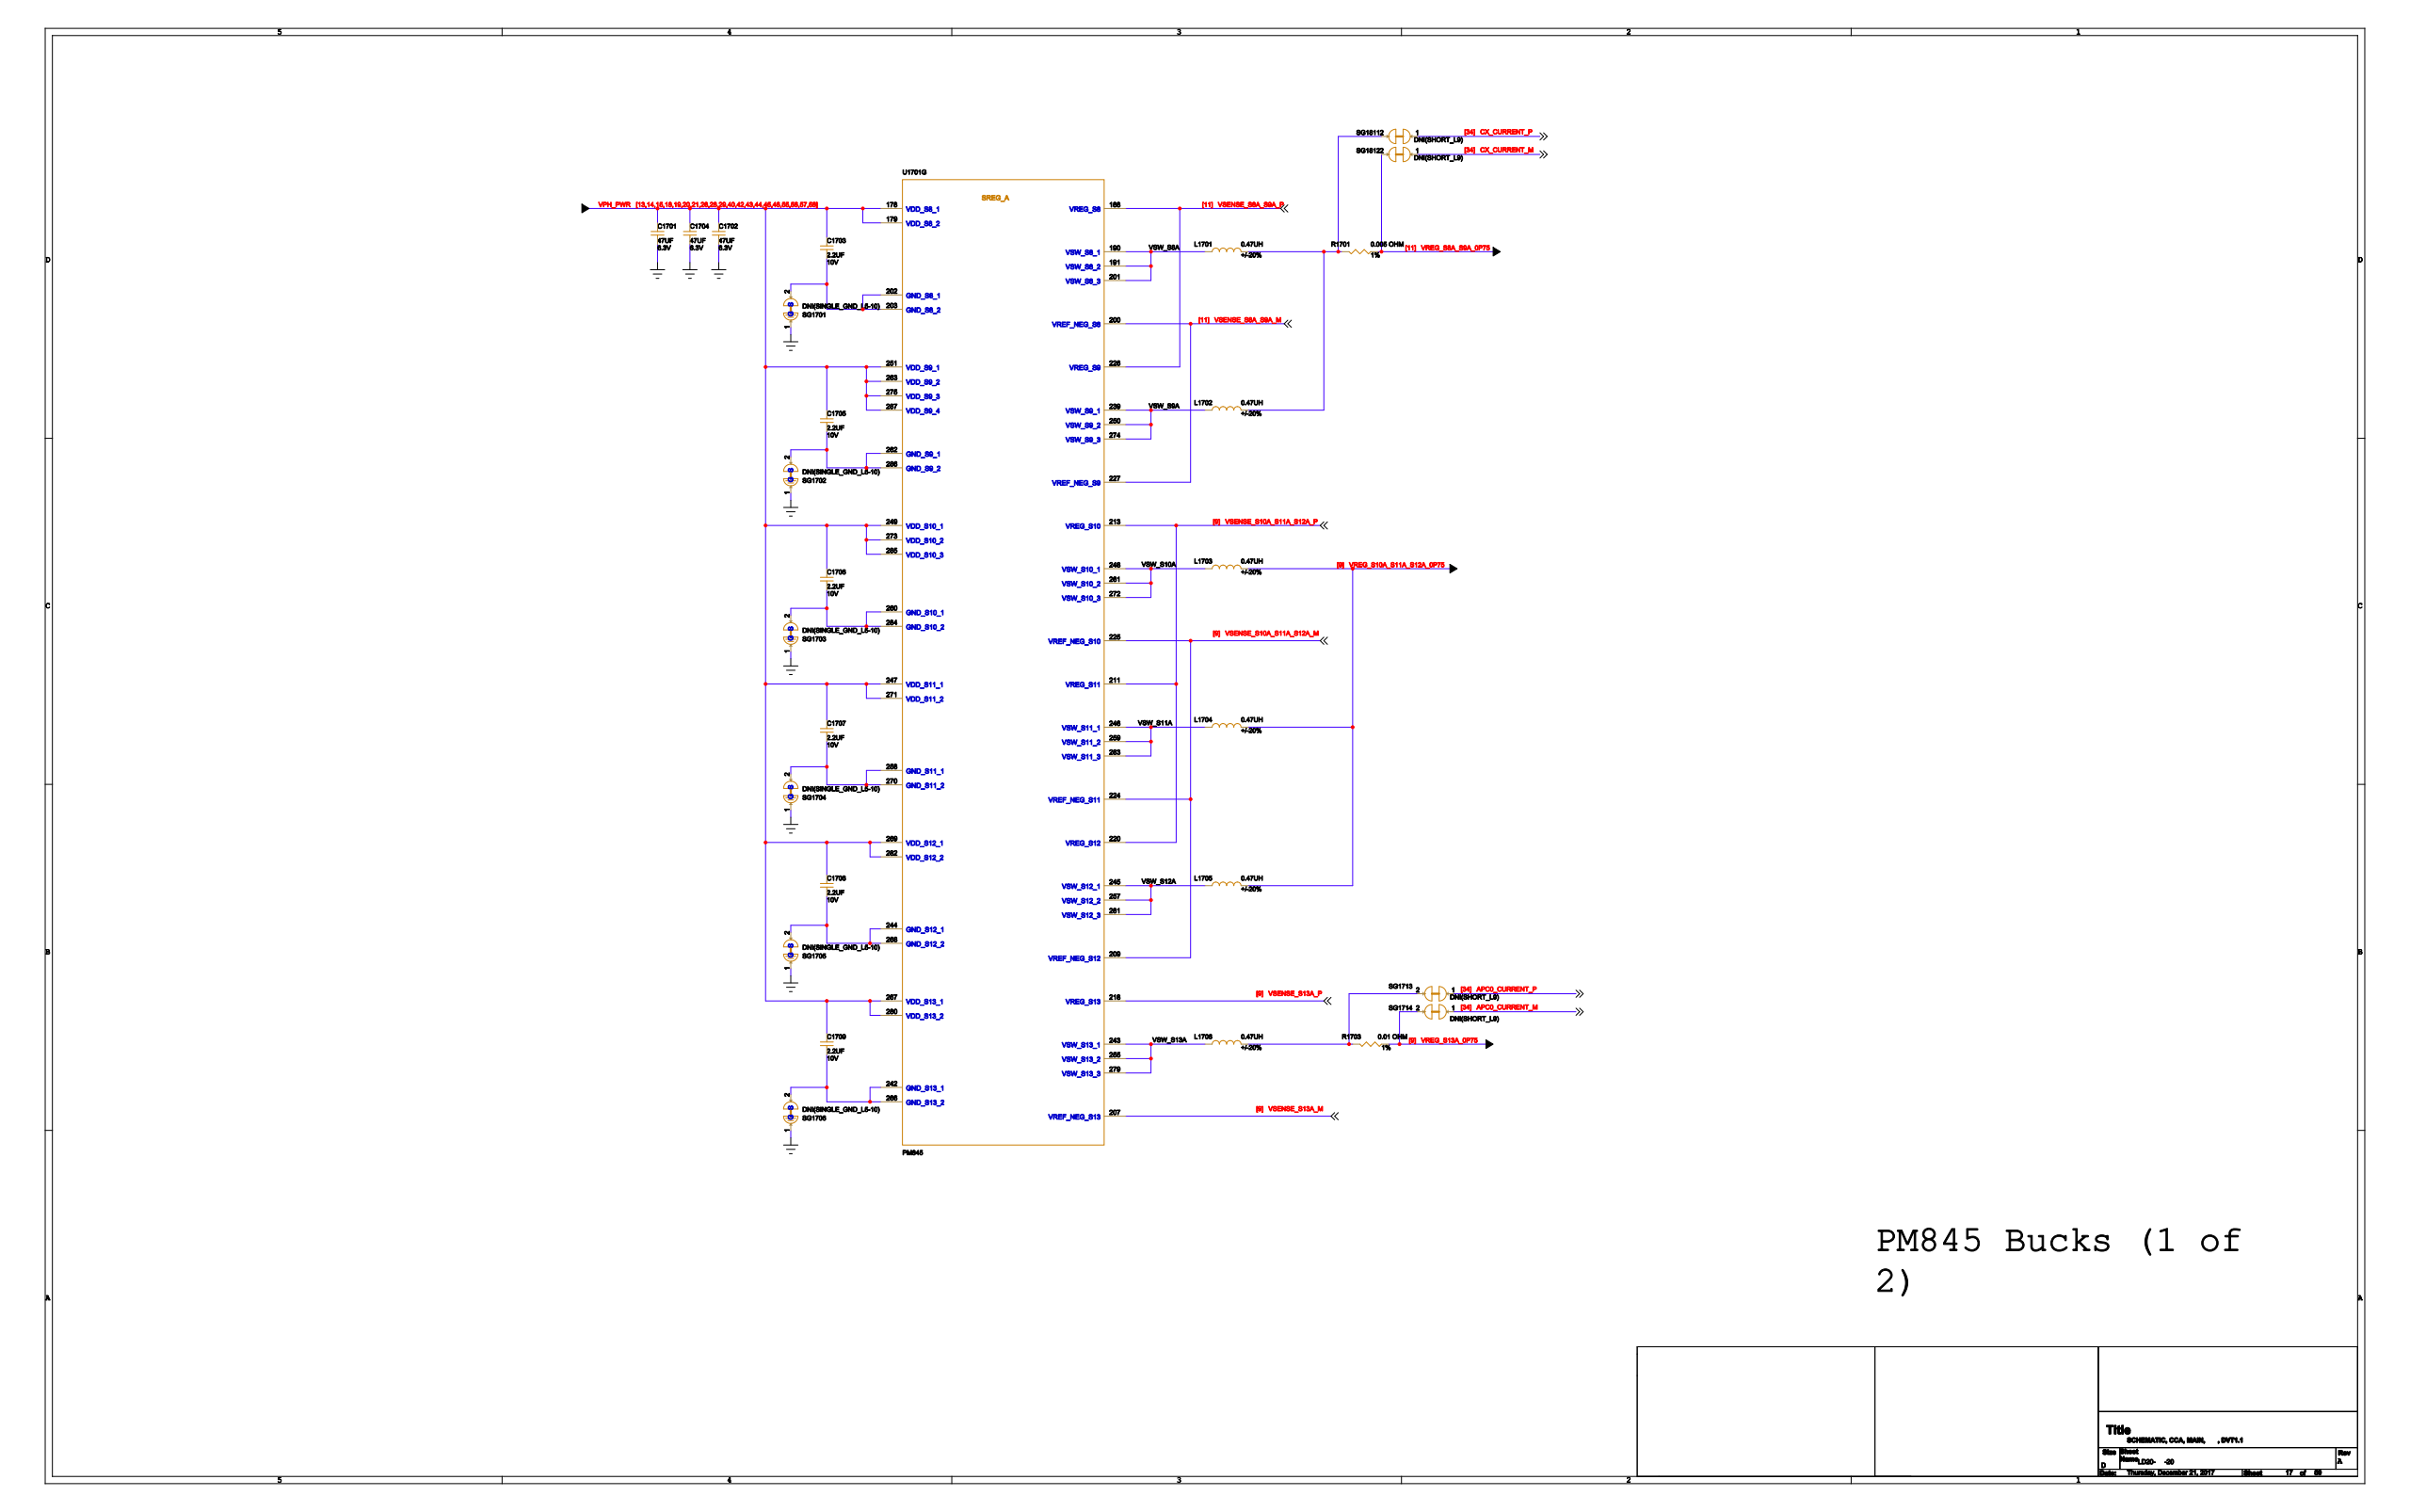Circuit board | Cadence Allegro | 1520 parts | 1149 nets | one sheet of the schematic
Parts on this sheet (reference | value | footprint):
C1701 | 47UF | 2P0603R
C1702 | 47UF | 2P0603R
C1703 | 2.2UF | 2P0201R
C1704 | 47UF | 2P0603R
C1705 | 2.2UF | 2P0201R
C1706 | 2.2UF | 2P0201R
C1707 | 2.2UF | 2P0201R
C1708 | 2.2UF | 2P0201R
C1709 | 2.2UF | 2P0201R
L1701 | 0.47UH | 2PSM87X71NV2
L1702 | 0.47UH | 2PSM87X71NV2
L1703 | 0.47UH | 2PSM87X71NV2
L1704 | 0.47UH | 2PSM87X71NV2
L1705 | 0.47UH | 2PSM87X71NV2
L1706 | 0.47UH | 2PSM87X71NV2
R1701 | 0.005 OHM | 2P0805R
R1703 | 0.01 OHM | 2P0603R
SG1701 | DNI(SINGLE_GND_L5-10) | GND_L5-10
SG1702 | DNI(SINGLE_GND_L5-10) | GND_L5-10
SG1703 | DNI(SINGLE_GND_L5-10) | GND_L5-10
SG1704 | DNI(SINGLE_GND_L5-10) | GND_L5-10
SG1705 | DNI(SINGLE_GND_L5-10) | GND_L5-10
SG1706 | DNI(SINGLE_GND_L5-10) | GND_L5-10
SG1713 | DNI(SHORT_L9) | SHORT_L9_2REC08X12
SG1714 | DNI(SHORT_L9) | SHORT_L9_2REC08X12
SG1811 | DNI(SHORT_L9) | SHORT_L9_2REC08X12
SG1812 | DNI(SHORT_L9) | SHORT_L9_2REC08X12
U1701 | PM845 | 287PGA242X240B138D45
Nets of these parts (net: part-pin ...):
GND: C1701-2 C1702-2 C1704-2 SG1701-1 SG1702-1 SG1703-1 SG1704-1 SG1705-1 SG1706-1
N34058891: C1703-2 SG1701-2 U1701-202 U1701-203
N34058962: C1705-2 SG1702-2 U1701-262 U1701-286
N34059057: C1706-2 SG1703-2 U1701-260 U1701-284
N34059143: C1707-2 SG1704-2 U1701-258 U1701-270
N34059235: C1708-2 SG1705-2 U1701-244 U1701-268
N34059323: C1709-2 SG1706-2 U1701-242 U1701-266
VPH_PWR: C1701-1 C1702-1 C1703-1 C1704-1 C1705-1 C1706-1 C1707-1 C1708-1 C1709-1 U1701-56 U1701-178 U1701-179 U1701-247 U1701-249 U1701-251 U1701-263 U1701-267 U1701-269 U1701-271 U1701-273 U1701-275 U1701-280 U1701-282 U1701-285 U1701-287
APC0_CURRENT_P: SG1713-1
N34910434: L1706-2 R1703-1 SG1713-2
APC0_CURRENT_M: SG1714-1
VREG_S13A_0P75: R1703-2 SG1714-2
CX_CURRENT_P: SG1811-1
N34439581: L1701-2 L1702-2 R1701-1 SG1811-2
CX_CURRENT_M: SG1812-1
VREG_S8A_S9A_0P75: R1701-2 SG1812-2
VREG_S10A_S11A_S12A_0P75: L1703-2 L1704-2 L1705-2
VSENSE_S10A_S11A_S12A_M: U1701-209 U1701-224 U1701-225
VSENSE_S10A_S11A_S12A_P: U1701-211 U1701-213 U1701-220
VSENSE_S13A_M: U1701-207
VSENSE_S13A_P: U1701-218
VSENSE_S8A_S9A_M: U1701-200 U1701-227
VSENSE_S8A_S9A_P: U1701-188 U1701-226
VSW_S8A: L1701-1 U1701-190 U1701-191 U1701-201
VSW_S9A: L1702-1 U1701-239 U1701-250 U1701-274
VSW_S10A: L1703-1 U1701-248 U1701-261 U1701-272
VSW_S11A: L1704-1 U1701-246 U1701-259 U1701-283
VSW_S12A: L1705-1 U1701-245 U1701-257 U1701-281
VSW_S13A: L1706-1 U1701-243 U1701-255 U1701-279